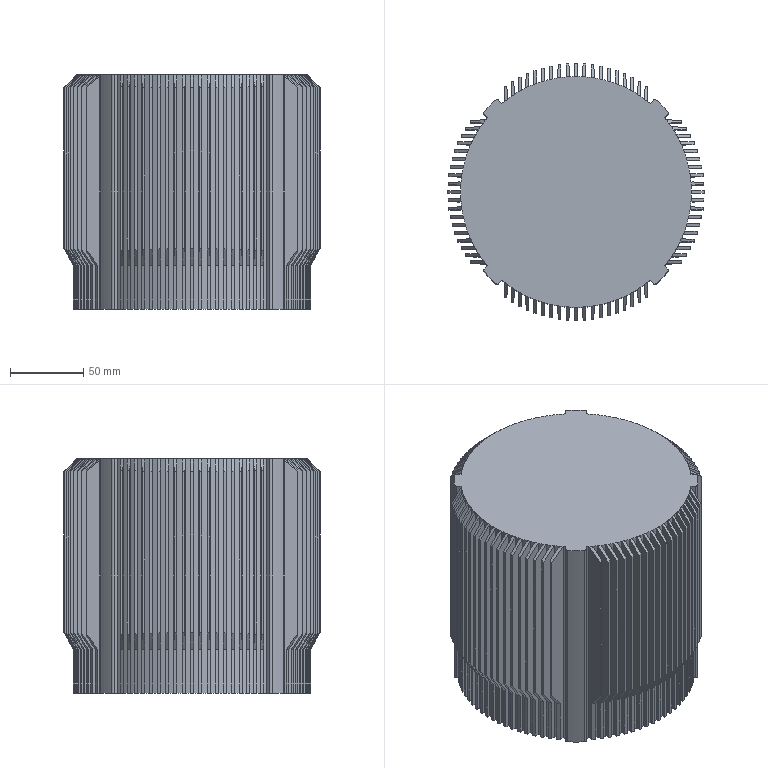Part | STEP file | Y2_JZ_80_B_1.step 1 | 1 solid | 558 faces | box 175 x 175 x 160 mm | volume 3332448 mm3 | cylinder 244 | plane 162 | cone 152 | commonest cylinder face diameters 157.5 x80 161.875 x76 175 x76 2.8 x8 166.25 x4